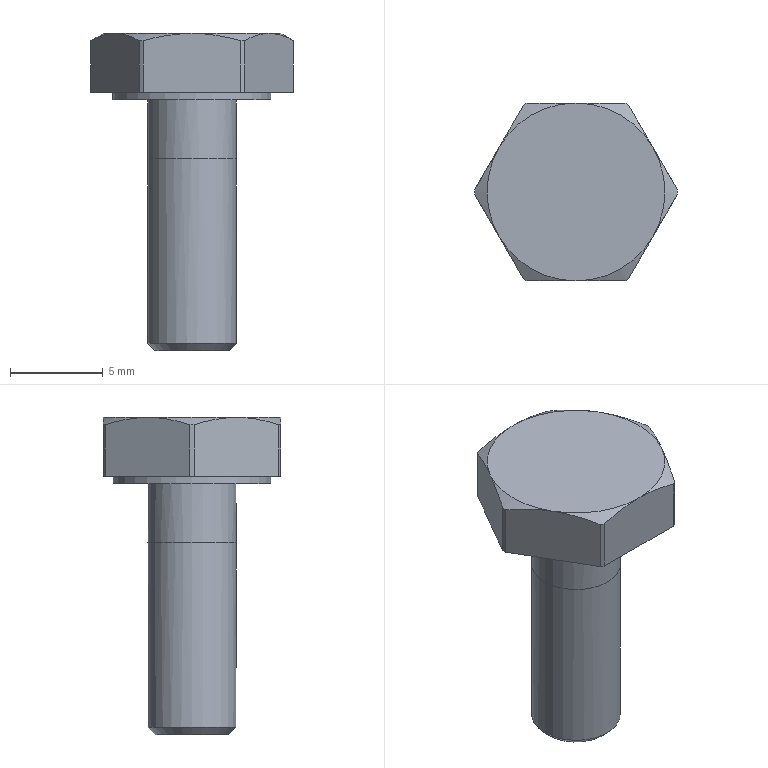Part | NX | features solid 2 | 1 solid | 26 faces | box 10.922 x 9.576 x 17.075 mm | volume 513.487 mm3 | plane 10 | cylinder 9 | cone 7 | commonest cylinder face diameters 10.922 x6 4.763 x2 8.509 x1
STEP:
#1=CARTESIAN_POINT('',(-2.381,0.,-3.581));
#2=VERTEX_POINT('',#1);
#3=CARTESIAN_POINT('',(0.,0.,-3.581));
#4=DIRECTION('',(0.,0.,-1.));
#5=DIRECTION('',(-1.,0.,0.));
#6=AXIS2_PLACEMENT_3D('',#3,#4,#5);
#7=CIRCLE('',#6,2.381);
#8=EDGE_CURVE('',#2,#2,#7,.T.);
#9=ORIENTED_EDGE('',*,*,#8,.T.);
#10=EDGE_LOOP('',(#9));
#11=FACE_BOUND('',#10,.T.);
#12=CARTESIAN_POINT('',(-2.381,0.,-6.756));
#13=VERTEX_POINT('',#12);
#14=CARTESIAN_POINT('',(-1.866,1.866,-6.756));
#15=CARTESIAN_POINT('',(-2.639,0.,-6.756));
#16=CARTESIAN_POINT('',(-1.866,-1.866,-6.756));
#17=CARTESIAN_POINT('',(0.,-2.639,-6.756));
#18=CARTESIAN_POINT('',(1.866,-1.866,-6.756));
#19=CARTESIAN_POINT('',(2.639,0.,-6.756));
#20=CARTESIAN_POINT('',(1.866,1.866,-6.756));
#21=CARTESIAN_POINT('',(0.,2.639,-6.756));
#22=CARTESIAN_POINT('',(-1.866,1.866,-6.756));
#23=CARTESIAN_POINT('',(-2.639,0.,-6.756));
#24=CARTESIAN_POINT('',(-1.866,-1.866,-6.756));
#25=B_SPLINE_CURVE_WITH_KNOTS('',3,(#14,#15,#16,#17,#18,#19,#20,#21,#22,#23,#24),.UNSPECIFIED.,.T.,.F.,(1,1,1,1,1,1,1,1,1,1,1,1,1,1,1),(-0.375,-0.25,-0.125,0.,0.125,0.25,0.375,0.5,0.625,0.75,0.875,1.,1.125,1.25,1.375),.UNSPECIFIED.);
#26=EDGE_CURVE('',#13,#13,#25,.T.);
#27=ORIENTED_EDGE('',*,*,#26,.T.);
#28=EDGE_LOOP('',(#27));
#29=FACE_BOUND('',#28,.T.);
#30=CARTESIAN_POINT('',(0.,0.,0.));
#31=DIRECTION('',(0.,0.,-1.));
#32=DIRECTION('',(-1.,0.,0.));
#33=AXIS2_PLACEMENT_3D('',#30,#31,#32);
#34=CYLINDRICAL_SURFACE('',#33,2.381);
#35=ADVANCED_FACE('',(#11,#29),#34,.T.);
#36=CARTESIAN_POINT('',(2.627,4.788,-3.175));
#37=VERTEX_POINT('',#36);
#38=CARTESIAN_POINT('',(2.833,4.669,-3.175));
#39=VERTEX_POINT('',#38);
#40=CARTESIAN_POINT('',(0.,0.,-3.175));
#41=DIRECTION('',(0.,0.,-1.));
#42=DIRECTION('',(-1.,0.,0.));
#43=AXIS2_PLACEMENT_3D('',#40,#41,#42);
#44=CIRCLE('',#43,5.461);
#45=EDGE_CURVE('',#37,#39,#44,.T.);
#46=ORIENTED_EDGE('',*,*,#45,.F.);
#47=CARTESIAN_POINT('',(2.627,4.788,-0.3886));
#48=VERTEX_POINT('',#47);
#49=CARTESIAN_POINT('',(2.627,4.788,0.));
#50=DIRECTION('',(0.,0.,-1.));
#51=VECTOR('',#50,1000.);
#52=LINE('',#49,#51);
#53=EDGE_CURVE('',#37,#48,#52,.F.);
#54=ORIENTED_EDGE('',*,*,#53,.T.);
#55=CARTESIAN_POINT('',(2.833,4.669,-0.3886));
#56=VERTEX_POINT('',#55);
#57=CARTESIAN_POINT('',(0.,0.,-0.3886));
#58=DIRECTION('',(0.,0.,-1.));
#59=DIRECTION('',(-1.,0.,0.));
#60=AXIS2_PLACEMENT_3D('',#57,#58,#59);
#61=CIRCLE('',#60,5.461);
#62=EDGE_CURVE('',#48,#56,#61,.T.);
#63=ORIENTED_EDGE('',*,*,#62,.T.);
#64=CARTESIAN_POINT('',(2.833,4.669,0.));
#65=DIRECTION('',(0.,0.,-1.));
#66=VECTOR('',#65,1000.);
#67=LINE('',#64,#66);
#68=EDGE_CURVE('',#56,#39,#67,.T.);
#69=ORIENTED_EDGE('',*,*,#68,.T.);
#70=EDGE_LOOP('',(#46,#54,#63,#69));
#71=FACE_BOUND('',#70,.T.);
#72=CARTESIAN_POINT('',(0.,0.,0.));
#73=DIRECTION('',(0.,0.,-1.));
#74=DIRECTION('',(-1.,0.,0.));
#75=AXIS2_PLACEMENT_3D('',#72,#73,#74);
#76=CYLINDRICAL_SURFACE('',#75,5.461);
#77=ADVANCED_FACE('',(#71),#76,.T.);
#78=CARTESIAN_POINT('',(-2.833,4.669,-0.3886));
#79=VERTEX_POINT('',#78);
#80=CARTESIAN_POINT('',(-2.627,4.788,-0.3886));
#81=VERTEX_POINT('',#80);
#82=CARTESIAN_POINT('',(0.,0.,-0.3886));
#83=DIRECTION('',(0.,0.,-1.));
#84=DIRECTION('',(-1.,0.,0.));
#85=AXIS2_PLACEMENT_3D('',#82,#83,#84);
#86=CIRCLE('',#85,5.461);
#87=EDGE_CURVE('',#79,#81,#86,.T.);
#88=ORIENTED_EDGE('',*,*,#87,.T.);
#89=CARTESIAN_POINT('',(-2.627,4.788,-3.175));
#90=VERTEX_POINT('',#89);
#91=CARTESIAN_POINT('',(-2.627,4.788,0.));
#92=DIRECTION('',(0.,0.,-1.));
#93=VECTOR('',#92,1000.);
#94=LINE('',#91,#93);
#95=EDGE_CURVE('',#81,#90,#94,.T.);
#96=ORIENTED_EDGE('',*,*,#95,.T.);
#97=CARTESIAN_POINT('',(-2.833,4.669,-3.175));
#98=VERTEX_POINT('',#97);
#99=CARTESIAN_POINT('',(0.,0.,-3.175));
#100=DIRECTION('',(0.,0.,-1.));
#101=DIRECTION('',(-1.,0.,0.));
#102=AXIS2_PLACEMENT_3D('',#99,#100,#101);
#103=CIRCLE('',#102,5.461);
#104=EDGE_CURVE('',#98,#90,#103,.T.);
#105=ORIENTED_EDGE('',*,*,#104,.F.);
#106=CARTESIAN_POINT('',(-2.833,4.669,0.));
#107=DIRECTION('',(0.,0.,-1.));
#108=VECTOR('',#107,1000.);
#109=LINE('',#106,#108);
#110=EDGE_CURVE('',#98,#79,#109,.F.);
#111=ORIENTED_EDGE('',*,*,#110,.T.);
#112=EDGE_LOOP('',(#88,#96,#105,#111));
#113=FACE_BOUND('',#112,.T.);
#114=CARTESIAN_POINT('',(0.,0.,0.));
#115=DIRECTION('',(0.,0.,-1.));
#116=DIRECTION('',(-1.,0.,0.));
#117=AXIS2_PLACEMENT_3D('',#114,#115,#116);
#118=CYLINDRICAL_SURFACE('',#117,5.461);
#119=ADVANCED_FACE('',(#113),#118,.T.);
#120=CARTESIAN_POINT('',(-5.46,-0.1193,-0.3886));
#121=VERTEX_POINT('',#120);
#122=CARTESIAN_POINT('',(-5.46,0.1193,-0.3886));
#123=VERTEX_POINT('',#122);
#124=CARTESIAN_POINT('',(0.,0.,-0.3886));
#125=DIRECTION('',(0.,0.,-1.));
#126=DIRECTION('',(-1.,0.,0.));
#127=AXIS2_PLACEMENT_3D('',#124,#125,#126);
#128=CIRCLE('',#127,5.461);
#129=EDGE_CURVE('',#121,#123,#128,.T.);
#130=ORIENTED_EDGE('',*,*,#129,.T.);
#131=CARTESIAN_POINT('',(-5.46,0.1193,-3.175));
#132=VERTEX_POINT('',#131);
#133=CARTESIAN_POINT('',(-5.46,0.1193,0.));
#134=DIRECTION('',(0.,0.,-1.));
#135=VECTOR('',#134,1000.);
#136=LINE('',#133,#135);
#137=EDGE_CURVE('',#123,#132,#136,.T.);
#138=ORIENTED_EDGE('',*,*,#137,.T.);
#139=CARTESIAN_POINT('',(-5.46,-0.1193,-3.175));
#140=VERTEX_POINT('',#139);
#141=CARTESIAN_POINT('',(0.,0.,-3.175));
#142=DIRECTION('',(0.,0.,-1.));
#143=DIRECTION('',(-1.,0.,0.));
#144=AXIS2_PLACEMENT_3D('',#141,#142,#143);
#145=CIRCLE('',#144,5.461);
#146=EDGE_CURVE('',#140,#132,#145,.T.);
#147=ORIENTED_EDGE('',*,*,#146,.F.);
#148=CARTESIAN_POINT('',(-5.46,-0.1193,0.));
#149=DIRECTION('',(0.,0.,-1.));
#150=VECTOR('',#149,1000.);
#151=LINE('',#148,#150);
#152=EDGE_CURVE('',#140,#121,#151,.F.);
#153=ORIENTED_EDGE('',*,*,#152,.T.);
#154=EDGE_LOOP('',(#130,#138,#147,#153));
#155=FACE_BOUND('',#154,.T.);
#156=CARTESIAN_POINT('',(0.,0.,0.));
#157=DIRECTION('',(0.,0.,-1.));
#158=DIRECTION('',(-1.,0.,0.));
#159=AXIS2_PLACEMENT_3D('',#156,#157,#158);
#160=CYLINDRICAL_SURFACE('',#159,5.461);
#161=ADVANCED_FACE('',(#155),#160,.T.);
#162=CARTESIAN_POINT('',(-2.627,-4.788,-0.3886));
#163=VERTEX_POINT('',#162);
#164=CARTESIAN_POINT('',(-2.833,-4.669,-0.3886));
#165=VERTEX_POINT('',#164);
#166=CARTESIAN_POINT('',(0.,0.,-0.3886));
#167=DIRECTION('',(0.,0.,-1.));
#168=DIRECTION('',(-1.,0.,0.));
#169=AXIS2_PLACEMENT_3D('',#166,#167,#168);
#170=CIRCLE('',#169,5.461);
#171=EDGE_CURVE('',#163,#165,#170,.T.);
#172=ORIENTED_EDGE('',*,*,#171,.T.);
#173=CARTESIAN_POINT('',(-2.833,-4.669,-3.175));
#174=VERTEX_POINT('',#173);
#175=CARTESIAN_POINT('',(-2.833,-4.669,0.));
#176=DIRECTION('',(0.,0.,-1.));
#177=VECTOR('',#176,1000.);
#178=LINE('',#175,#177);
#179=EDGE_CURVE('',#165,#174,#178,.T.);
#180=ORIENTED_EDGE('',*,*,#179,.T.);
#181=CARTESIAN_POINT('',(-2.627,-4.788,-3.175));
#182=VERTEX_POINT('',#181);
#183=CARTESIAN_POINT('',(0.,0.,-3.175));
#184=DIRECTION('',(0.,0.,-1.));
#185=DIRECTION('',(-1.,0.,0.));
#186=AXIS2_PLACEMENT_3D('',#183,#184,#185);
#187=CIRCLE('',#186,5.461);
#188=EDGE_CURVE('',#182,#174,#187,.T.);
#189=ORIENTED_EDGE('',*,*,#188,.F.);
#190=CARTESIAN_POINT('',(-2.627,-4.788,0.));
#191=DIRECTION('',(0.,0.,-1.));
#192=VECTOR('',#191,1000.);
#193=LINE('',#190,#192);
#194=EDGE_CURVE('',#182,#163,#193,.F.);
#195=ORIENTED_EDGE('',*,*,#194,.T.);
#196=EDGE_LOOP('',(#172,#180,#189,#195));
#197=FACE_BOUND('',#196,.T.);
#198=CARTESIAN_POINT('',(0.,0.,0.));
#199=DIRECTION('',(0.,0.,-1.));
#200=DIRECTION('',(-1.,0.,0.));
#201=AXIS2_PLACEMENT_3D('',#198,#199,#200);
#202=CYLINDRICAL_SURFACE('',#201,5.461);
#203=ADVANCED_FACE('',(#197),#202,.T.);
#204=CARTESIAN_POINT('',(2.833,-4.669,-0.3886));
#205=VERTEX_POINT('',#204);
#206=CARTESIAN_POINT('',(2.627,-4.788,-0.3886));
#207=VERTEX_POINT('',#206);
#208=CARTESIAN_POINT('',(0.,0.,-0.3886));
#209=DIRECTION('',(0.,0.,-1.));
#210=DIRECTION('',(-1.,0.,0.));
#211=AXIS2_PLACEMENT_3D('',#208,#209,#210);
#212=CIRCLE('',#211,5.461);
#213=EDGE_CURVE('',#205,#207,#212,.T.);
#214=ORIENTED_EDGE('',*,*,#213,.T.);
#215=CARTESIAN_POINT('',(2.627,-4.788,-3.175));
#216=VERTEX_POINT('',#215);
#217=CARTESIAN_POINT('',(2.627,-4.788,0.));
#218=DIRECTION('',(0.,0.,-1.));
#219=VECTOR('',#218,1000.);
#220=LINE('',#217,#219);
#221=EDGE_CURVE('',#207,#216,#220,.T.);
#222=ORIENTED_EDGE('',*,*,#221,.T.);
#223=CARTESIAN_POINT('',(2.833,-4.669,-3.175));
#224=VERTEX_POINT('',#223);
#225=CARTESIAN_POINT('',(0.,0.,-3.175));
#226=DIRECTION('',(0.,0.,-1.));
#227=DIRECTION('',(-1.,0.,0.));
#228=AXIS2_PLACEMENT_3D('',#225,#226,#227);
#229=CIRCLE('',#228,5.461);
#230=EDGE_CURVE('',#224,#216,#229,.T.);
#231=ORIENTED_EDGE('',*,*,#230,.F.);
#232=CARTESIAN_POINT('',(2.833,-4.669,0.));
#233=DIRECTION('',(0.,0.,-1.));
#234=VECTOR('',#233,1000.);
#235=LINE('',#232,#234);
#236=EDGE_CURVE('',#224,#205,#235,.F.);
#237=ORIENTED_EDGE('',*,*,#236,.T.);
#238=EDGE_LOOP('',(#214,#222,#231,#237));
#239=FACE_BOUND('',#238,.T.);
#240=CARTESIAN_POINT('',(0.,0.,0.));
#241=DIRECTION('',(0.,0.,-1.));
#242=DIRECTION('',(-1.,0.,0.));
#243=AXIS2_PLACEMENT_3D('',#240,#241,#242);
#244=CYLINDRICAL_SURFACE('',#243,5.461);
#245=ADVANCED_FACE('',(#239),#244,.T.);
#246=ORIENTED_EDGE('',*,*,#62,.F.);
#247=CARTESIAN_POINT('',(0.,4.788,0.));
#248=VERTEX_POINT('',#247);
#249=CARTESIAN_POINT('',(0.,4.788,0.));
#250=CARTESIAN_POINT('',(0.8868,4.788,0.));
#251=CARTESIAN_POINT('',(1.776,4.788,-0.1525));
#252=CARTESIAN_POINT('',(2.627,4.788,-0.3886));
#253=B_SPLINE_CURVE_WITH_KNOTS('',3,(#249,#250,#251,#252),.UNSPECIFIED.,.F.,.F.,(4,4),(0.007722,0.01038),.UNSPECIFIED.);
#254=EDGE_CURVE('',#48,#248,#253,.F.);
#255=ORIENTED_EDGE('',*,*,#254,.T.);
#256=CARTESIAN_POINT('',(4.146,2.394,0.));
#257=VERTEX_POINT('',#256);
#258=CARTESIAN_POINT('',(0.,0.,0.));
#259=DIRECTION('',(0.,0.,-1.));
#260=DIRECTION('',(-1.,0.,0.));
#261=AXIS2_PLACEMENT_3D('',#258,#259,#260);
#262=CIRCLE('',#261,4.788);
#263=EDGE_CURVE('',#248,#257,#262,.T.);
#264=ORIENTED_EDGE('',*,*,#263,.T.);
#265=CARTESIAN_POINT('',(4.146,2.394,0.));
#266=CARTESIAN_POINT('',(3.703,3.163,0.));
#267=CARTESIAN_POINT('',(3.262,3.925,-0.1503));
#268=CARTESIAN_POINT('',(2.833,4.669,-0.3886));
#269=B_SPLINE_CURVE_WITH_KNOTS('',3,(#265,#266,#267,#268),.UNSPECIFIED.,.F.,.F.,(4,4),(0.002655,0.005296),.UNSPECIFIED.);
#270=EDGE_CURVE('',#257,#56,#269,.T.);
#271=ORIENTED_EDGE('',*,*,#270,.T.);
#272=EDGE_LOOP('',(#246,#255,#264,#271));
#273=FACE_BOUND('',#272,.T.);
#274=CARTESIAN_POINT('',(0.,0.,-0.3886));
#275=DIRECTION('',(0.,0.,-1.));
#276=DIRECTION('',(-1.,0.,0.));
#277=AXIS2_PLACEMENT_3D('',#274,#275,#276);
#278=CONICAL_SURFACE('',#277,5.461,1.047);
#279=ADVANCED_FACE('',(#273),#278,.T.);
#280=CARTESIAN_POINT('',(-4.146,2.394,0.));
#281=VERTEX_POINT('',#280);
#282=CARTESIAN_POINT('',(0.,0.,0.));
#283=DIRECTION('',(0.,0.,-1.));
#284=DIRECTION('',(-1.,0.,0.));
#285=AXIS2_PLACEMENT_3D('',#282,#283,#284);
#286=CIRCLE('',#285,4.788);
#287=EDGE_CURVE('',#281,#248,#286,.T.);
#288=ORIENTED_EDGE('',*,*,#287,.T.);
#289=CARTESIAN_POINT('',(-2.627,4.788,-0.3886));
#290=CARTESIAN_POINT('',(-1.77,4.788,-0.1508));
#291=CARTESIAN_POINT('',(-0.8866,4.788,0.));
#292=CARTESIAN_POINT('',(0.,4.788,0.));
#293=B_SPLINE_CURVE_WITH_KNOTS('',3,(#289,#290,#291,#292),.UNSPECIFIED.,.F.,.F.,(4,4),(0.005068,0.007722),.UNSPECIFIED.);
#294=EDGE_CURVE('',#248,#81,#293,.F.);
#295=ORIENTED_EDGE('',*,*,#294,.T.);
#296=ORIENTED_EDGE('',*,*,#87,.F.);
#297=CARTESIAN_POINT('',(-2.833,4.669,-0.3886));
#298=CARTESIAN_POINT('',(-3.264,3.923,-0.1495));
#299=CARTESIAN_POINT('',(-3.7,3.167,0.));
#300=CARTESIAN_POINT('',(-4.146,2.394,0.));
#301=B_SPLINE_CURVE_WITH_KNOTS('',3,(#297,#298,#299,#300),.UNSPECIFIED.,.F.,.F.,(4,4),(0.00000074,0.002655),.UNSPECIFIED.);
#302=EDGE_CURVE('',#79,#281,#301,.T.);
#303=ORIENTED_EDGE('',*,*,#302,.T.);
#304=EDGE_LOOP('',(#288,#295,#296,#303));
#305=FACE_BOUND('',#304,.T.);
#306=CARTESIAN_POINT('',(0.,0.,-0.3886));
#307=DIRECTION('',(0.,0.,-1.));
#308=DIRECTION('',(-1.,0.,0.));
#309=AXIS2_PLACEMENT_3D('',#306,#307,#308);
#310=CONICAL_SURFACE('',#309,5.461,1.047);
#311=ADVANCED_FACE('',(#305),#310,.T.);
#312=CARTESIAN_POINT('',(-4.146,-2.394,0.));
#313=VERTEX_POINT('',#312);
#314=CARTESIAN_POINT('',(0.,0.,0.));
#315=DIRECTION('',(0.,0.,-1.));
#316=DIRECTION('',(-1.,0.,0.));
#317=AXIS2_PLACEMENT_3D('',#314,#315,#316);
#318=CIRCLE('',#317,4.788);
#319=EDGE_CURVE('',#313,#281,#318,.T.);
#320=ORIENTED_EDGE('',*,*,#319,.T.);
#321=CARTESIAN_POINT('',(-4.146,2.394,0.));
#322=CARTESIAN_POINT('',(-4.59,1.625,0.));
#323=CARTESIAN_POINT('',(-5.031,0.8625,-0.1503));
#324=CARTESIAN_POINT('',(-5.46,0.1193,-0.3886));
#325=B_SPLINE_CURVE_WITH_KNOTS('',3,(#321,#322,#323,#324),.UNSPECIFIED.,.F.,.F.,(4,4),(0.002655,0.005296),.UNSPECIFIED.);
#326=EDGE_CURVE('',#281,#123,#325,.T.);
#327=ORIENTED_EDGE('',*,*,#326,.T.);
#328=ORIENTED_EDGE('',*,*,#129,.F.);
#329=CARTESIAN_POINT('',(-5.46,-0.1193,-0.3886));
#330=CARTESIAN_POINT('',(-5.029,-0.8651,-0.1495));
#331=CARTESIAN_POINT('',(-4.593,-1.621,0.));
#332=CARTESIAN_POINT('',(-4.146,-2.394,0.));
#333=B_SPLINE_CURVE_WITH_KNOTS('',3,(#329,#330,#331,#332),.UNSPECIFIED.,.F.,.F.,(4,4),(0.00000074,0.002655),.UNSPECIFIED.);
#334=EDGE_CURVE('',#121,#313,#333,.T.);
#335=ORIENTED_EDGE('',*,*,#334,.T.);
#336=EDGE_LOOP('',(#320,#327,#328,#335));
#337=FACE_BOUND('',#336,.T.);
#338=CARTESIAN_POINT('',(0.,0.,-0.3886));
#339=DIRECTION('',(0.,0.,-1.));
#340=DIRECTION('',(-1.,0.,0.));
#341=AXIS2_PLACEMENT_3D('',#338,#339,#340);
#342=CONICAL_SURFACE('',#341,5.461,1.047);
#343=ADVANCED_FACE('',(#337),#342,.T.);
#344=CARTESIAN_POINT('',(0.,-4.788,0.));
#345=VERTEX_POINT('',#344);
#346=CARTESIAN_POINT('',(0.,0.,0.));
#347=DIRECTION('',(0.,0.,-1.));
#348=DIRECTION('',(-1.,0.,0.));
#349=AXIS2_PLACEMENT_3D('',#346,#347,#348);
#350=CIRCLE('',#349,4.788);
#351=EDGE_CURVE('',#345,#313,#350,.T.);
#352=ORIENTED_EDGE('',*,*,#351,.T.);
#353=CARTESIAN_POINT('',(-4.146,-2.394,0.));
#354=CARTESIAN_POINT('',(-3.703,-3.163,0.));
#355=CARTESIAN_POINT('',(-3.262,-3.925,-0.1503));
#356=CARTESIAN_POINT('',(-2.833,-4.669,-0.3886));
#357=B_SPLINE_CURVE_WITH_KNOTS('',3,(#353,#354,#355,#356),.UNSPECIFIED.,.F.,.F.,(4,4),(0.002655,0.005296),.UNSPECIFIED.);
#358=EDGE_CURVE('',#313,#165,#357,.T.);
#359=ORIENTED_EDGE('',*,*,#358,.T.);
#360=ORIENTED_EDGE('',*,*,#171,.F.);
#361=CARTESIAN_POINT('',(-2.627,-4.788,-0.3886));
#362=CARTESIAN_POINT('',(-1.77,-4.788,-0.1508));
#363=CARTESIAN_POINT('',(-0.8866,-4.788,0.));
#364=CARTESIAN_POINT('',(0.,-4.788,0.));
#365=B_SPLINE_CURVE_WITH_KNOTS('',3,(#361,#362,#363,#364),.UNSPECIFIED.,.F.,.F.,(4,4),(0.005068,0.007722),.UNSPECIFIED.);
#366=EDGE_CURVE('',#163,#345,#365,.T.);
#367=ORIENTED_EDGE('',*,*,#366,.T.);
#368=EDGE_LOOP('',(#352,#359,#360,#367));
#369=FACE_BOUND('',#368,.T.);
#370=CARTESIAN_POINT('',(0.,0.,-0.3886));
#371=DIRECTION('',(0.,0.,-1.));
#372=DIRECTION('',(-1.,0.,0.));
#373=AXIS2_PLACEMENT_3D('',#370,#371,#372);
#374=CONICAL_SURFACE('',#373,5.461,1.047);
#375=ADVANCED_FACE('',(#369),#374,.T.);
#376=CARTESIAN_POINT('',(4.146,-2.394,0.));
#377=VERTEX_POINT('',#376);
#378=CARTESIAN_POINT('',(0.,0.,0.));
#379=DIRECTION('',(0.,0.,-1.));
#380=DIRECTION('',(-1.,0.,0.));
#381=AXIS2_PLACEMENT_3D('',#378,#379,#380);
#382=CIRCLE('',#381,4.788);
#383=EDGE_CURVE('',#377,#345,#382,.T.);
#384=ORIENTED_EDGE('',*,*,#383,.T.);
#385=CARTESIAN_POINT('',(0.,-4.788,0.));
#386=CARTESIAN_POINT('',(0.8868,-4.788,0.));
#387=CARTESIAN_POINT('',(1.776,-4.788,-0.1525));
#388=CARTESIAN_POINT('',(2.627,-4.788,-0.3886));
#389=B_SPLINE_CURVE_WITH_KNOTS('',3,(#385,#386,#387,#388),.UNSPECIFIED.,.F.,.F.,(4,4),(0.007722,0.01038),.UNSPECIFIED.);
#390=EDGE_CURVE('',#345,#207,#389,.T.);
#391=ORIENTED_EDGE('',*,*,#390,.T.);
#392=ORIENTED_EDGE('',*,*,#213,.F.);
#393=CARTESIAN_POINT('',(2.833,-4.669,-0.3886));
#394=CARTESIAN_POINT('',(3.264,-3.923,-0.1495));
#395=CARTESIAN_POINT('',(3.7,-3.167,0.));
#396=CARTESIAN_POINT('',(4.146,-2.394,0.));
#397=B_SPLINE_CURVE_WITH_KNOTS('',3,(#393,#394,#395,#396),.UNSPECIFIED.,.F.,.F.,(4,4),(0.00000074,0.002655),.UNSPECIFIED.);
#398=EDGE_CURVE('',#205,#377,#397,.T.);
#399=ORIENTED_EDGE('',*,*,#398,.T.);
#400=EDGE_LOOP('',(#384,#391,#392,#399));
#401=FACE_BOUND('',#400,.T.);
#402=CARTESIAN_POINT('',(0.,0.,-0.3886));
#403=DIRECTION('',(0.,0.,-1.));
#404=DIRECTION('',(-1.,0.,0.));
#405=AXIS2_PLACEMENT_3D('',#402,#403,#404);
#406=CONICAL_SURFACE('',#405,5.461,1.047);
#407=ADVANCED_FACE('',(#401),#406,.T.);
#408=ORIENTED_EDGE('',*,*,#104,.T.);
#409=CARTESIAN_POINT('',(4.255,4.788,-3.175));
#410=DIRECTION('',(1.,0.,0.));
#411=VECTOR('',#410,1000.);
#412=LINE('',#409,#411);
#413=EDGE_CURVE('',#90,#37,#412,.T.);
#414=ORIENTED_EDGE('',*,*,#413,.T.);
#415=ORIENTED_EDGE('',*,*,#45,.T.);
#416=CARTESIAN_POINT('',(5.46,0.1193,-3.175));
#417=VERTEX_POINT('',#416);
#418=CARTESIAN_POINT('',(5.21,0.5517,-3.175));
#419=DIRECTION('',(0.5,-0.866,0.));
#420=VECTOR('',#419,1000.);
#421=LINE('',#418,#420);
#422=EDGE_CURVE('',#39,#417,#421,.T.);
#423=ORIENTED_EDGE('',*,*,#422,.T.);
#424=CARTESIAN_POINT('',(5.46,-0.1193,-3.175));
#425=VERTEX_POINT('',#424);
#426=CARTESIAN_POINT('',(0.,0.,-3.175));
#427=DIRECTION('',(0.,0.,-1.));
#428=DIRECTION('',(-1.,0.,0.));
#429=AXIS2_PLACEMENT_3D('',#426,#427,#428);
#430=CIRCLE('',#429,5.461);
#431=EDGE_CURVE('',#417,#425,#430,.T.);
#432=ORIENTED_EDGE('',*,*,#431,.T.);
#433=CARTESIAN_POINT('',(5.21,-0.5517,-3.175));
#434=DIRECTION('',(-0.5,-0.866,0.));
#435=VECTOR('',#434,1000.);
#436=LINE('',#433,#435);
#437=EDGE_CURVE('',#425,#224,#436,.T.);
#438=ORIENTED_EDGE('',*,*,#437,.T.);
#439=ORIENTED_EDGE('',*,*,#230,.T.);
#440=CARTESIAN_POINT('',(4.255,-4.788,-3.175));
#441=DIRECTION('',(-1.,0.,0.));
#442=VECTOR('',#441,1000.);
#443=LINE('',#440,#442);
#444=EDGE_CURVE('',#216,#182,#443,.T.);
#445=ORIENTED_EDGE('',*,*,#444,.T.);
#446=ORIENTED_EDGE('',*,*,#188,.T.);
#447=CARTESIAN_POINT('',(-3.083,-4.236,-3.175));
#448=DIRECTION('',(-0.5,0.866,0.));
#449=VECTOR('',#448,1000.);
#450=LINE('',#447,#449);
#451=EDGE_CURVE('',#174,#140,#450,.T.);
#452=ORIENTED_EDGE('',*,*,#451,.T.);
#453=ORIENTED_EDGE('',*,*,#146,.T.);
#454=CARTESIAN_POINT('',(-3.083,4.236,-3.175));
#455=DIRECTION('',(0.5,0.866,0.));
#456=VECTOR('',#455,1000.);
#457=LINE('',#454,#456);
#458=EDGE_CURVE('',#132,#98,#457,.T.);
#459=ORIENTED_EDGE('',*,*,#458,.T.);
#460=EDGE_LOOP('',(#408,#414,#415,#423,#432,#438,#439,#445,#446,#452,#453,#459));
#461=FACE_BOUND('',#460,.T.);
#462=CARTESIAN_POINT('',(-4.255,0.,-3.175));
#463=VERTEX_POINT('',#462);
#464=CARTESIAN_POINT('',(0.,0.,-3.175));
#465=DIRECTION('',(0.,0.,-1.));
#466=DIRECTION('',(-1.,0.,0.));
#467=AXIS2_PLACEMENT_3D('',#464,#465,#466);
#468=CIRCLE('',#467,4.255);
#469=EDGE_CURVE('',#463,#463,#468,.T.);
#470=ORIENTED_EDGE('',*,*,#469,.F.);
#471=EDGE_LOOP('',(#470));
#472=FACE_BOUND('',#471,.T.);
#473=CARTESIAN_POINT('',(4.255,0.,-3.175));
#474=DIRECTION('',(0.,0.,-1.));
#475=DIRECTION('',(-1.,0.,0.));
#476=AXIS2_PLACEMENT_3D('',#473,#474,#475);
#477=PLANE('',#476);
#478=ADVANCED_FACE('',(#461,#472),#477,.T.);
#479=CARTESIAN_POINT('',(5.46,0.1193,-0.3886));
#480=VERTEX_POINT('',#479);
#481=CARTESIAN_POINT('',(5.46,-0.1193,-0.3886));
#482=VERTEX_POINT('',#481);
#483=CARTESIAN_POINT('',(0.,0.,-0.3886));
#484=DIRECTION('',(0.,0.,-1.));
#485=DIRECTION('',(-1.,0.,0.));
#486=AXIS2_PLACEMENT_3D('',#483,#484,#485);
#487=CIRCLE('',#486,5.461);
#488=EDGE_CURVE('',#480,#482,#487,.T.);
#489=ORIENTED_EDGE('',*,*,#488,.T.);
#490=CARTESIAN_POINT('',(5.46,-0.1193,0.));
#491=DIRECTION('',(0.,0.,-1.));
#492=VECTOR('',#491,1000.);
#493=LINE('',#490,#492);
#494=EDGE_CURVE('',#482,#425,#493,.T.);
#495=ORIENTED_EDGE('',*,*,#494,.T.);
#496=ORIENTED_EDGE('',*,*,#431,.F.);
#497=CARTESIAN_POINT('',(5.46,0.1193,0.));
#498=DIRECTION('',(0.,0.,-1.));
#499=VECTOR('',#498,1000.);
#500=LINE('',#497,#499);
#501=EDGE_CURVE('',#417,#480,#500,.F.);
#502=ORIENTED_EDGE('',*,*,#501,.T.);
#503=EDGE_LOOP('',(#489,#495,#496,#502));
#504=FACE_BOUND('',#503,.T.);
#505=CARTESIAN_POINT('',(0.,0.,0.));
#506=DIRECTION('',(0.,0.,-1.));
#507=DIRECTION('',(-1.,0.,0.));
#508=AXIS2_PLACEMENT_3D('',#505,#506,#507);
#509=CYLINDRICAL_SURFACE('',#508,5.461);
#510=ADVANCED_FACE('',(#504),#509,.T.);
#511=CARTESIAN_POINT('',(0.,0.,0.));
#512=DIRECTION('',(0.,0.,-1.));
#513=DIRECTION('',(-1.,0.,0.));
#514=AXIS2_PLACEMENT_3D('',#511,#512,#513);
#515=CIRCLE('',#514,4.788);
#516=EDGE_CURVE('',#257,#377,#515,.T.);
#517=ORIENTED_EDGE('',*,*,#516,.T.);
#518=CARTESIAN_POINT('',(4.146,-2.394,0.));
#519=CARTESIAN_POINT('',(4.59,-1.625,0.));
#520=CARTESIAN_POINT('',(5.031,-0.8625,-0.1503));
#521=CARTESIAN_POINT('',(5.46,-0.1193,-0.3886));
#522=B_SPLINE_CURVE_WITH_KNOTS('',3,(#518,#519,#520,#521),.UNSPECIFIED.,.F.,.F.,(4,4),(0.002655,0.005296),.UNSPECIFIED.);
#523=EDGE_CURVE('',#377,#482,#522,.T.);
#524=ORIENTED_EDGE('',*,*,#523,.T.);
#525=ORIENTED_EDGE('',*,*,#488,.F.);
#526=CARTESIAN_POINT('',(5.46,0.1193,-0.3886));
#527=CARTESIAN_POINT('',(5.029,0.8651,-0.1495));
#528=CARTESIAN_POINT('',(4.593,1.621,0.));
#529=CARTESIAN_POINT('',(4.146,2.394,0.));
#530=B_SPLINE_CURVE_WITH_KNOTS('',3,(#526,#527,#528,#529),.UNSPECIFIED.,.F.,.F.,(4,4),(0.00000074,0.002655),.UNSPECIFIED.);
#531=EDGE_CURVE('',#480,#257,#530,.T.);
#532=ORIENTED_EDGE('',*,*,#531,.T.);
#533=EDGE_LOOP('',(#517,#524,#525,#532));
#534=FACE_BOUND('',#533,.T.);
#535=CARTESIAN_POINT('',(0.,0.,-0.3886));
#536=DIRECTION('',(0.,0.,-1.));
#537=DIRECTION('',(-1.,0.,0.));
#538=AXIS2_PLACEMENT_3D('',#535,#536,#537);
#539=CONICAL_SURFACE('',#538,5.461,1.047);
#540=ADVANCED_FACE('',(#534),#539,.T.);
#541=ORIENTED_EDGE('',*,*,#287,.F.);
#542=ORIENTED_EDGE('',*,*,#319,.F.);
#543=ORIENTED_EDGE('',*,*,#351,.F.);
#544=ORIENTED_EDGE('',*,*,#383,.F.);
#545=ORIENTED_EDGE('',*,*,#516,.F.);
#546=ORIENTED_EDGE('',*,*,#263,.F.);
#547=EDGE_LOOP('',(#541,#542,#543,#544,#545,#546));
#548=FACE_BOUND('',#547,.T.);
#549=CARTESIAN_POINT('',(4.788,0.,0.));
#550=DIRECTION('',(0.,0.,1.));
#551=DIRECTION('',(1.,0.,0.));
#552=AXIS2_PLACEMENT_3D('',#549,#550,#551);
#553=PLANE('',#552);
#554=ADVANCED_FACE('',(#548),#553,.T.);
#555=CARTESIAN_POINT('',(-2.,0.,-17.075));
#556=VERTEX_POINT('',#555);
#557=CARTESIAN_POINT('',(0.,0.,-17.075));
#558=DIRECTION('',(0.,0.,-1.));
#559=DIRECTION('',(-1.,0.,0.));
#560=AXIS2_PLACEMENT_3D('',#557,#558,#559);
#561=CIRCLE('',#560,2.);
#562=EDGE_CURVE('',#556,#556,#561,.T.);
#563=ORIENTED_EDGE('',*,*,#562,.T.);
#564=EDGE_LOOP('',(#563));
#565=FACE_BOUND('',#564,.T.);
#566=CARTESIAN_POINT('',(0.,0.,-17.075));
#567=DIRECTION('',(0.,0.,-1.));
#568=DIRECTION('',(-1.,0.,0.));
#569=AXIS2_PLACEMENT_3D('',#566,#567,#568);
#570=PLANE('',#569);
#571=ADVANCED_FACE('',(#565),#570,.T.);
#572=CARTESIAN_POINT('',(-2.381,0.,-16.694));
#573=VERTEX_POINT('',#572);
#574=CARTESIAN_POINT('',(0.,0.,-16.694));
#575=DIRECTION('',(0.,0.,-1.));
#576=DIRECTION('',(-1.,0.,0.));
#577=AXIS2_PLACEMENT_3D('',#574,#575,#576);
#578=CIRCLE('',#577,2.381);
#579=EDGE_CURVE('',#573,#573,#578,.T.);
#580=ORIENTED_EDGE('',*,*,#579,.T.);
#581=EDGE_LOOP('',(#580));
#582=FACE_BOUND('',#581,.T.);
#583=ORIENTED_EDGE('',*,*,#562,.F.);
#584=EDGE_LOOP('',(#583));
#585=FACE_BOUND('',#584,.T.);
#586=CARTESIAN_POINT('',(0.,0.,-17.075));
#587=DIRECTION('',(0.,0.,1.));
#588=DIRECTION('',(1.,0.,0.));
#589=AXIS2_PLACEMENT_3D('',#586,#587,#588);
#590=CONICAL_SURFACE('',#589,2.,0.7854);
#591=ADVANCED_FACE('',(#582,#585),#590,.T.);
#592=ORIENTED_EDGE('',*,*,#26,.F.);
#593=EDGE_LOOP('',(#592));
#594=FACE_BOUND('',#593,.T.);
#595=ORIENTED_EDGE('',*,*,#579,.F.);
#596=EDGE_LOOP('',(#595));
#597=FACE_BOUND('',#596,.T.);
#598=CARTESIAN_POINT('',(0.,0.,0.));
#599=DIRECTION('',(0.,0.,-1.));
#600=DIRECTION('',(-1.,0.,0.));
#601=AXIS2_PLACEMENT_3D('',#598,#599,#600);
#602=CYLINDRICAL_SURFACE('',#601,2.381);
#603=ADVANCED_FACE('',(#594,#597),#602,.T.);
#604=CARTESIAN_POINT('',(-4.255,0.,-3.581));
#605=VERTEX_POINT('',#604);
#606=CARTESIAN_POINT('',(0.,0.,-3.581));
#607=DIRECTION('',(0.,0.,-1.));
#608=DIRECTION('',(-1.,0.,0.));
#609=AXIS2_PLACEMENT_3D('',#606,#607,#608);
#610=CIRCLE('',#609,4.255);
#611=EDGE_CURVE('',#605,#605,#610,.T.);
#612=ORIENTED_EDGE('',*,*,#611,.T.);
#613=EDGE_LOOP('',(#612));
#614=FACE_BOUND('',#613,.T.);
#615=ORIENTED_EDGE('',*,*,#8,.F.);
#616=EDGE_LOOP('',(#615));
#617=FACE_BOUND('',#616,.T.);
#618=CARTESIAN_POINT('',(2.381,0.,-3.581));
#619=DIRECTION('',(0.,0.,-1.));
#620=DIRECTION('',(-1.,0.,0.));
#621=AXIS2_PLACEMENT_3D('',#618,#619,#620);
#622=PLANE('',#621);
#623=ADVANCED_FACE('',(#614,#617),#622,.T.);
#624=ORIENTED_EDGE('',*,*,#469,.T.);
#625=EDGE_LOOP('',(#624));
#626=FACE_BOUND('',#625,.T.);
#627=ORIENTED_EDGE('',*,*,#611,.F.);
#628=EDGE_LOOP('',(#627));
#629=FACE_BOUND('',#628,.T.);
#630=CARTESIAN_POINT('',(0.,0.,0.));
#631=DIRECTION('',(0.,0.,-1.));
#632=DIRECTION('',(-1.,0.,0.));
#633=AXIS2_PLACEMENT_3D('',#630,#631,#632);
#634=CYLINDRICAL_SURFACE('',#633,4.255);
#635=ADVANCED_FACE('',(#626,#629),#634,.T.);
#636=ORIENTED_EDGE('',*,*,#422,.F.);
#637=ORIENTED_EDGE('',*,*,#68,.F.);
#638=ORIENTED_EDGE('',*,*,#270,.F.);
#639=ORIENTED_EDGE('',*,*,#531,.F.);
#640=ORIENTED_EDGE('',*,*,#501,.F.);
#641=EDGE_LOOP('',(#636,#637,#638,#639,#640));
#642=FACE_BOUND('',#641,.T.);
#643=CARTESIAN_POINT('',(5.529,0.,-18.783));
#644=DIRECTION('',(0.866,0.5,0.));
#645=DIRECTION('',(-0.5,0.866,0.));
#646=AXIS2_PLACEMENT_3D('',#643,#644,#645);
#647=PLANE('',#646);
#648=ADVANCED_FACE('',(#642),#647,.T.);
#649=ORIENTED_EDGE('',*,*,#437,.F.);
#650=ORIENTED_EDGE('',*,*,#494,.F.);
#651=ORIENTED_EDGE('',*,*,#523,.F.);
#652=ORIENTED_EDGE('',*,*,#398,.F.);
#653=ORIENTED_EDGE('',*,*,#236,.F.);
#654=EDGE_LOOP('',(#649,#650,#651,#652,#653));
#655=FACE_BOUND('',#654,.T.);
#656=CARTESIAN_POINT('',(2.764,-4.788,-18.783));
#657=DIRECTION('',(0.866,-0.5,0.));
#658=DIRECTION('',(0.5,0.866,0.));
#659=AXIS2_PLACEMENT_3D('',#656,#657,#658);
#660=PLANE('',#659);
#661=ADVANCED_FACE('',(#655),#660,.T.);
#662=ORIENTED_EDGE('',*,*,#444,.F.);
#663=ORIENTED_EDGE('',*,*,#221,.F.);
#664=ORIENTED_EDGE('',*,*,#390,.F.);
#665=ORIENTED_EDGE('',*,*,#366,.F.);
#666=ORIENTED_EDGE('',*,*,#194,.F.);
#667=EDGE_LOOP('',(#662,#663,#664,#665,#666));
#668=FACE_BOUND('',#667,.T.);
#669=CARTESIAN_POINT('',(-2.764,-4.788,-18.783));
#670=DIRECTION('',(0.,-1.,0.));
#671=DIRECTION('',(0.,0.,-1.));
#672=AXIS2_PLACEMENT_3D('',#669,#670,#671);
#673=PLANE('',#672);
#674=ADVANCED_FACE('',(#668),#673,.T.);
#675=ORIENTED_EDGE('',*,*,#451,.F.);
#676=ORIENTED_EDGE('',*,*,#179,.F.);
#677=ORIENTED_EDGE('',*,*,#358,.F.);
#678=ORIENTED_EDGE('',*,*,#334,.F.);
#679=ORIENTED_EDGE('',*,*,#152,.F.);
#680=EDGE_LOOP('',(#675,#676,#677,#678,#679));
#681=FACE_BOUND('',#680,.T.);
#682=CARTESIAN_POINT('',(-5.529,0.,-18.783));
#683=DIRECTION('',(-0.866,-0.5,0.));
#684=DIRECTION('',(0.5,-0.866,0.));
#685=AXIS2_PLACEMENT_3D('',#682,#683,#684);
#686=PLANE('',#685);
#687=ADVANCED_FACE('',(#681),#686,.T.);
#688=ORIENTED_EDGE('',*,*,#458,.F.);
#689=ORIENTED_EDGE('',*,*,#137,.F.);
#690=ORIENTED_EDGE('',*,*,#326,.F.);
#691=ORIENTED_EDGE('',*,*,#302,.F.);
#692=ORIENTED_EDGE('',*,*,#110,.F.);
#693=EDGE_LOOP('',(#688,#689,#690,#691,#692));
#694=FACE_BOUND('',#693,.T.);
#695=CARTESIAN_POINT('',(-2.764,4.788,-18.783));
#696=DIRECTION('',(-0.866,0.5,0.));
#697=DIRECTION('',(-0.5,-0.866,0.));
#698=AXIS2_PLACEMENT_3D('',#695,#696,#697);
#699=PLANE('',#698);
#700=ADVANCED_FACE('',(#694),#699,.T.);
#701=ORIENTED_EDGE('',*,*,#413,.F.);
#702=ORIENTED_EDGE('',*,*,#95,.F.);
#703=ORIENTED_EDGE('',*,*,#294,.F.);
#704=ORIENTED_EDGE('',*,*,#254,.F.);
#705=ORIENTED_EDGE('',*,*,#53,.F.);
#706=EDGE_LOOP('',(#701,#702,#703,#704,#705));
#707=FACE_BOUND('',#706,.T.);
#708=CARTESIAN_POINT('',(2.764,4.788,-18.783));
#709=DIRECTION('',(0.,1.,0.));
#710=DIRECTION('',(0.,0.,1.));
#711=AXIS2_PLACEMENT_3D('',#708,#709,#710);
#712=PLANE('',#711);
#713=ADVANCED_FACE('',(#707),#712,.T.);
#714=CLOSED_SHELL('',(#35,#77,#119,#161,#203,#245,#279,#311,#343,#375,#407,#478,#510,#540,#554,#571,#591,#603,#623,#635,#648,#661,#674,#687,#700,#713));
#715=MANIFOLD_SOLID_BREP('',#714);
#716=(LENGTH_UNIT()NAMED_UNIT(*)SI_UNIT(.MILLI.,.METRE.));
#717=UNCERTAINTY_MEASURE_WITH_UNIT(LENGTH_MEASURE(0.0508),#716,'','');
#718=(NAMED_UNIT(*)PLANE_ANGLE_UNIT()SI_UNIT($,.RADIAN.));
#719=(NAMED_UNIT(*)SI_UNIT($,.STERADIAN.)SOLID_ANGLE_UNIT());
#720=(GEOMETRIC_REPRESENTATION_CONTEXT(3)GLOBAL_UNCERTAINTY_ASSIGNED_CONTEXT((#717))GLOBAL_UNIT_ASSIGNED_CONTEXT((#716,#718,#719))REPRESENTATION_CONTEXT('',''));
#721=ADVANCED_BREP_SHAPE_REPRESENTATION('',(#715),#720);